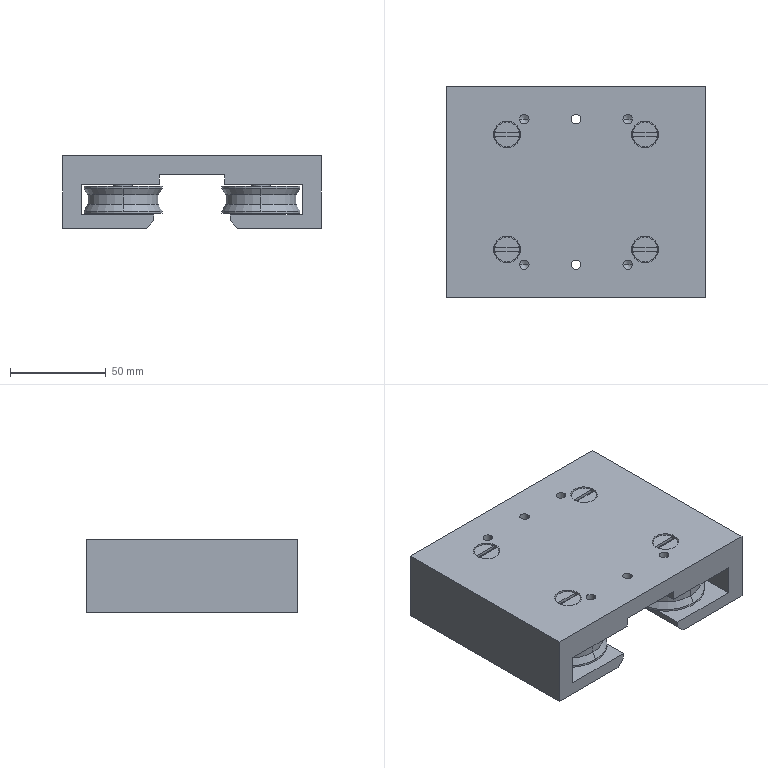Part | SolidWorks | features ReferencePattern 15, LocalLPattern 1 | 21 solids | 1460 faces | box 135 x 110 x 38 mm | volume 364943 mm3 | sphere 576 | torus 304 | plane 280 | cylinder 244 | cone 56 | commonest cylinder face diameters 22 x40 10 x32 13.5 x32 18.5 x32 11 x16 15.127 x16